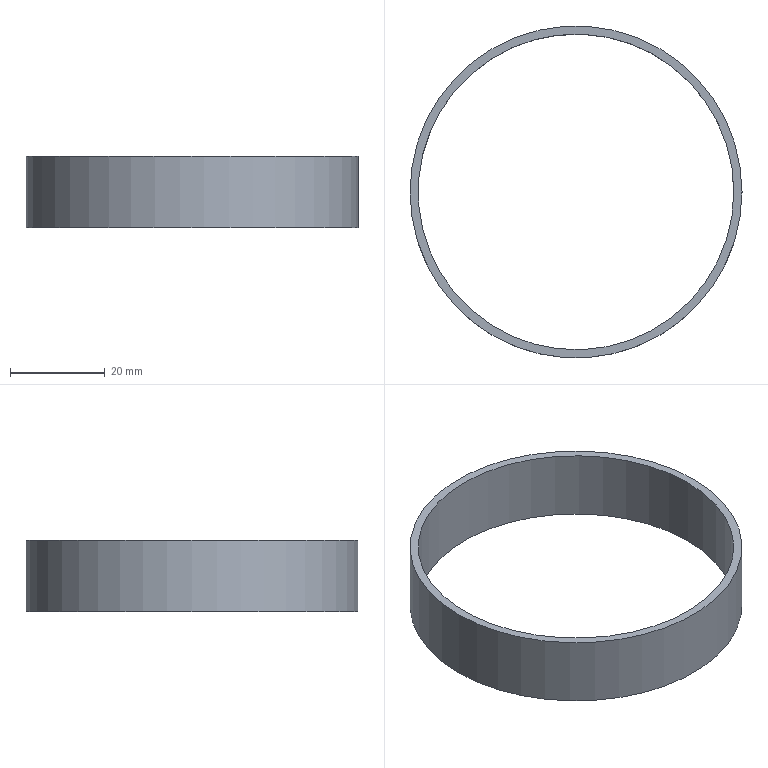Part | NX | features solid 2 | 1 solid | 4 faces | box 69.911 x 69.911 x 15 mm | volume 5557 mm3 | cylinder 2 | plane 2 | commonest cylinder face diameters 66.451 x1 69.911 x1
STEP:
#1=CARTESIAN_POINT('',(-46.774,-440.,-196.));
#2=VERTEX_POINT('',#1);
#3=CARTESIAN_POINT('',(-80.,-440.,-196.));
#4=DIRECTION('',(0.,0.,1.));
#5=DIRECTION('',(1.,0.,0.));
#6=AXIS2_PLACEMENT_3D('',#3,#4,#5);
#7=CIRCLE('',#6,33.226);
#8=EDGE_CURVE('',#2,#2,#7,.T.);
#9=ORIENTED_EDGE('',*,*,#8,.F.);
#10=EDGE_LOOP('',(#9));
#11=FACE_BOUND('',#10,.T.);
#12=CARTESIAN_POINT('',(-46.774,-440.,-181.));
#13=VERTEX_POINT('',#12);
#14=CARTESIAN_POINT('',(-80.,-440.,-181.));
#15=DIRECTION('',(0.,0.,1.));
#16=DIRECTION('',(1.,0.,0.));
#17=AXIS2_PLACEMENT_3D('',#14,#15,#16);
#18=CIRCLE('',#17,33.226);
#19=EDGE_CURVE('',#13,#13,#18,.T.);
#20=ORIENTED_EDGE('',*,*,#19,.T.);
#21=EDGE_LOOP('',(#20));
#22=FACE_BOUND('',#21,.T.);
#23=CARTESIAN_POINT('',(-80.,-440.,-196.));
#24=DIRECTION('',(0.,0.,1.));
#25=DIRECTION('',(-1.,0.,0.));
#26=AXIS2_PLACEMENT_3D('',#23,#24,#25);
#27=CYLINDRICAL_SURFACE('',#26,33.226);
#28=ADVANCED_FACE('',(#11,#22),#27,.F.);
#29=CARTESIAN_POINT('',(-45.045,-440.,-196.));
#30=VERTEX_POINT('',#29);
#31=CARTESIAN_POINT('',(-80.,-440.,-196.));
#32=DIRECTION('',(0.,0.,1.));
#33=DIRECTION('',(1.,0.,0.));
#34=AXIS2_PLACEMENT_3D('',#31,#32,#33);
#35=CIRCLE('',#34,34.955);
#36=EDGE_CURVE('',#30,#30,#35,.T.);
#37=ORIENTED_EDGE('',*,*,#36,.T.);
#38=EDGE_LOOP('',(#37));
#39=FACE_BOUND('',#38,.T.);
#40=CARTESIAN_POINT('',(-45.045,-440.,-181.));
#41=VERTEX_POINT('',#40);
#42=CARTESIAN_POINT('',(-80.,-440.,-181.));
#43=DIRECTION('',(0.,0.,1.));
#44=DIRECTION('',(1.,0.,0.));
#45=AXIS2_PLACEMENT_3D('',#42,#43,#44);
#46=CIRCLE('',#45,34.955);
#47=EDGE_CURVE('',#41,#41,#46,.T.);
#48=ORIENTED_EDGE('',*,*,#47,.F.);
#49=EDGE_LOOP('',(#48));
#50=FACE_BOUND('',#49,.T.);
#51=CARTESIAN_POINT('',(-80.,-440.,-196.));
#52=DIRECTION('',(0.,0.,1.));
#53=DIRECTION('',(-1.,0.,0.));
#54=AXIS2_PLACEMENT_3D('',#51,#52,#53);
#55=CYLINDRICAL_SURFACE('',#54,34.955);
#56=ADVANCED_FACE('',(#39,#50),#55,.T.);
#57=ORIENTED_EDGE('',*,*,#8,.T.);
#58=EDGE_LOOP('',(#57));
#59=FACE_BOUND('',#58,.T.);
#60=ORIENTED_EDGE('',*,*,#36,.F.);
#61=EDGE_LOOP('',(#60));
#62=FACE_BOUND('',#61,.T.);
#63=CARTESIAN_POINT('',(-80.,-440.,-196.));
#64=DIRECTION('',(0.,0.,-1.));
#65=DIRECTION('',(1.,0.,0.));
#66=AXIS2_PLACEMENT_3D('',#63,#64,#65);
#67=PLANE('',#66);
#68=ADVANCED_FACE('',(#59,#62),#67,.T.);
#69=ORIENTED_EDGE('',*,*,#19,.F.);
#70=EDGE_LOOP('',(#69));
#71=FACE_BOUND('',#70,.T.);
#72=ORIENTED_EDGE('',*,*,#47,.T.);
#73=EDGE_LOOP('',(#72));
#74=FACE_BOUND('',#73,.T.);
#75=CARTESIAN_POINT('',(-80.,-440.,-181.));
#76=DIRECTION('',(0.,0.,-1.));
#77=DIRECTION('',(1.,0.,0.));
#78=AXIS2_PLACEMENT_3D('',#75,#76,#77);
#79=PLANE('',#78);
#80=ADVANCED_FACE('',(#71,#74),#79,.F.);
#81=CLOSED_SHELL('',(#28,#56,#68,#80));
#82=MANIFOLD_SOLID_BREP('',#81);
#83=(LENGTH_UNIT()NAMED_UNIT(*)SI_UNIT(.MILLI.,.METRE.));
#84=UNCERTAINTY_MEASURE_WITH_UNIT(LENGTH_MEASURE(0.00001),#83,'','');
#85=(NAMED_UNIT(*)PLANE_ANGLE_UNIT()SI_UNIT($,.RADIAN.));
#86=(NAMED_UNIT(*)SI_UNIT($,.STERADIAN.)SOLID_ANGLE_UNIT());
#87=(GEOMETRIC_REPRESENTATION_CONTEXT(3)GLOBAL_UNCERTAINTY_ASSIGNED_CONTEXT((#84))GLOBAL_UNIT_ASSIGNED_CONTEXT((#83,#85,#86))REPRESENTATION_CONTEXT('',''));
#88=ADVANCED_BREP_SHAPE_REPRESENTATION('',(#82),#87);